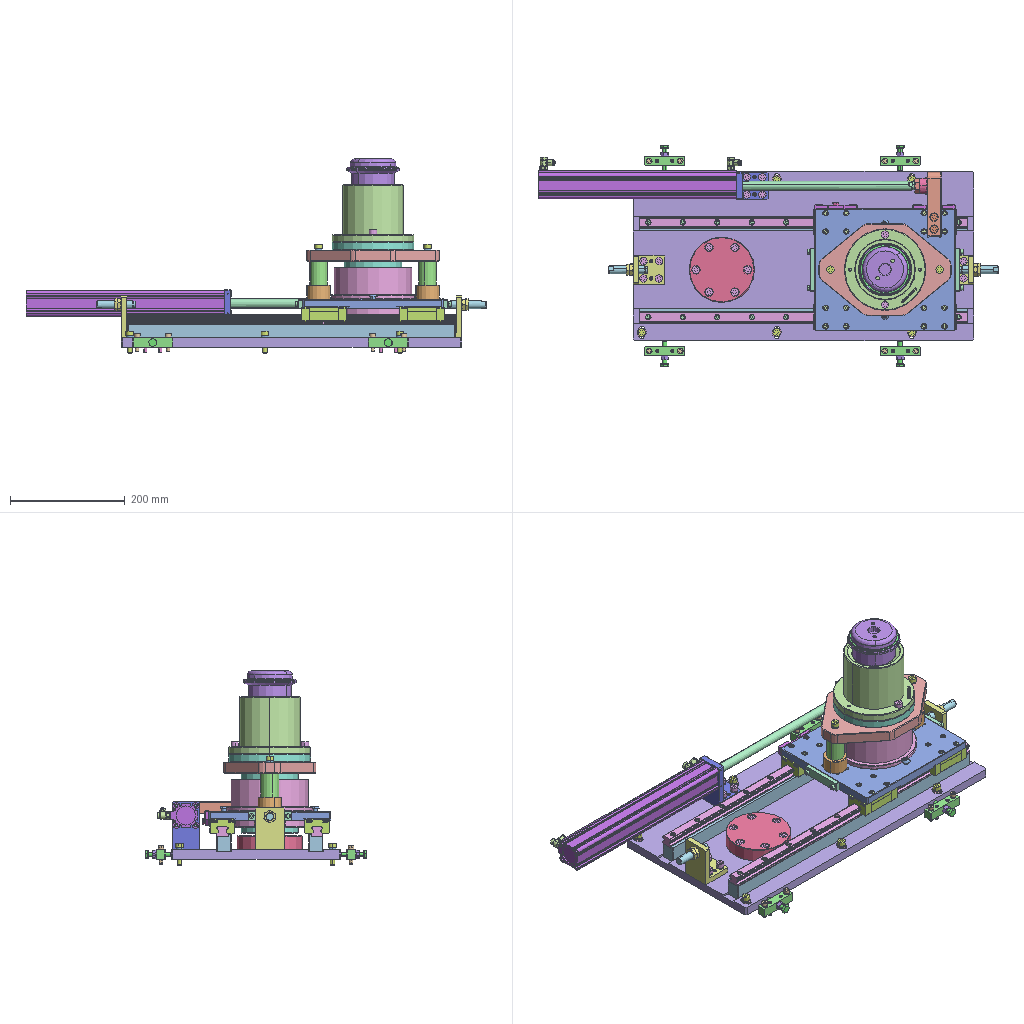Assembly | SolidWorks | 63 different items | 324 placed | box 801 x 386 x 338 mm
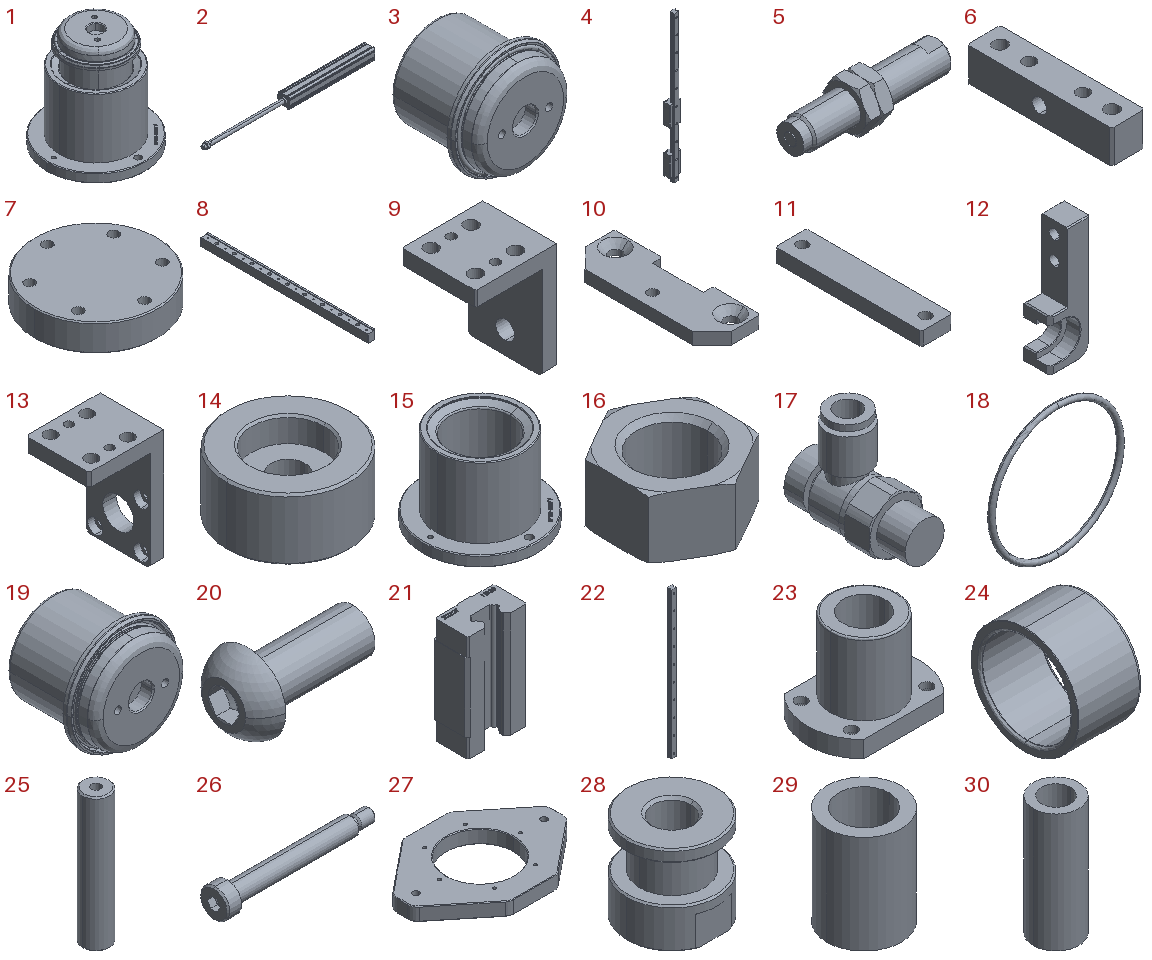Parts list (item | name | quantity | parent item | size | volume | features):
1 | (subassembly) | x1 | - | 142 x 142 x 150.5 mm | 760859 mm3 | -
2 | (subassembly) | x1 | - | 676 x 49.5 x 45 mm | 398264 mm3 | -
3 | (subassembly) | x1 | in 1 | 92 x 83 x 92 mm | 149578 mm3 | -
4 | (subassembly) | x2 | - | 44 x 30 x 570 mm | 296416 mm3 | -
5 | (subassembly) | x2 | - | 67.1 x 21.939 x 19.79 mm | 12290 mm3 | -
6 | - | x4 | - | 16 x 70 x 16 mm | 15307 mm3 | features HoleWzd 3, Chamfer 1, ExtruThin 1
7 | - | x1 | - | 114 x 114 x 25 mm | 237134 mm3 | features Chamfer 1, CirPattern 1, Extrusion 1, HoleWzd 1
8 | - | x2 | - | 25 x 570 x 30 mm | 386551 mm3 | features Chamfer 2, HoleWzd 2, Extrusion 1, ICE 1, LPattern 1
9 | - | x2 | - | 55 x 50 x 73 mm | 54613 mm3 | features HoleWzd 3, Chamfer 2, Extrusion 1, ICE 1
10 | - | x2 | - | 25 x 75 x 6 mm | 9049 mm3 | features Chamfer 3, HoleWzd 2, ExtruThin 1, ICE 1
11 | - | x2 | - | 16 x 75 x 7 mm | 8053 mm3 | features Chamfer 1, Extrusion 1, HoleWzd 1
12 | - | x1 | - | 36 x 24 x 110 mm | 50408 mm3 | features Chamfer 7, ICE 3, Extrusion 1, Fillet 1, HoleWzd 1
13 | - | x1 | - | 55 x 47 x 84 mm | 50700 mm3 | features HoleWzd 3, Chamfer 2, ICE 2, CirPattern 1, Extrusion 1
14 | - | x1 | in 1 | 30 x 30 x 15 mm | 8651 mm3 | features Chamfer 2, ICE 2, Extrusion 1
15 | - | x1 | in 1 | 142 x 142 x 106 mm | 593458 mm3 | features ICE 5, Chamfer 4, Fillet 3, HoleWzd 3, Extrusion 1, RevCut 1
16 | - | x4 | - | 12.482 x 14.38 x 6.8 mm | 562.42 mm3 | features Cut 2, Chamfer 1, Extrusion 1
17 | - | x2 | - | 13 x 29.2 x 26.1 mm | 3843 mm3 | features BaseBody 1
18 | - | x1 | in 3 | 86.03 x 3.53 x 86.03 mm | 2537 mm3 | features RefAxis 1, Revolution 1
19 | - | x1 | in 3 | 92 x 83 x 92 mm | 147042 mm3 | features Fillet 7, ICE 5, Chamfer 3, RevCut 3, CirPattern 1, Revolution 1
20 | - | x2 | - | 24.4 x 14 x 14 mm | 1421 mm3 | features RevCut 2, Revolution 2, Cut 1, LPattern 1, RefAxis 1
21 | - | x4 | in 4 | 44 x 25.4 x 77.8 mm | 67305 mm3 | features BaseBody 1
22 | - | x2 | in 4 | 20 x 17.5 x 570 mm | 161806 mm3 | features ICE 2, BaseBody 1, HoleWzd 1, LPattern 1
23 | - | x2 | - | 54 x 38 x 42 mm | 27501 mm3 | features BaseBody 1
24 | - | x1 | - | 70 x 120 x 120 mm | 240473 mm3 | features BaseBody 1
25 | - | x2 | - | 20 x 20 x 100 mm | 29690 mm3 | features Chamfer 2, HoleWzd 2, Extrusion 1
26 | - | x1 | in 1 | 70 x 13 x 13 mm | 3701 mm3 | features BaseBody 1
27 | - | x1 | - | 230 x 160 x 20 mm | 361707 mm3 | features Chamfer 3, HoleWzd 2, ICE 2, Cut 1, Extrusion 1, Fillet 1
28 | - | x1 | - | 29.5 x 29.5 x 29 mm | 12018 mm3 | features BaseBody 1
29 | - | x2 | - | 31 x 31 x 41 mm | 16745 mm3 | features Extrusion 1
30 | - | x1 | in 1 | 16.5 x 16.5 x 43 mm | 5471 mm3 | features Extrusion 1, ICE 1
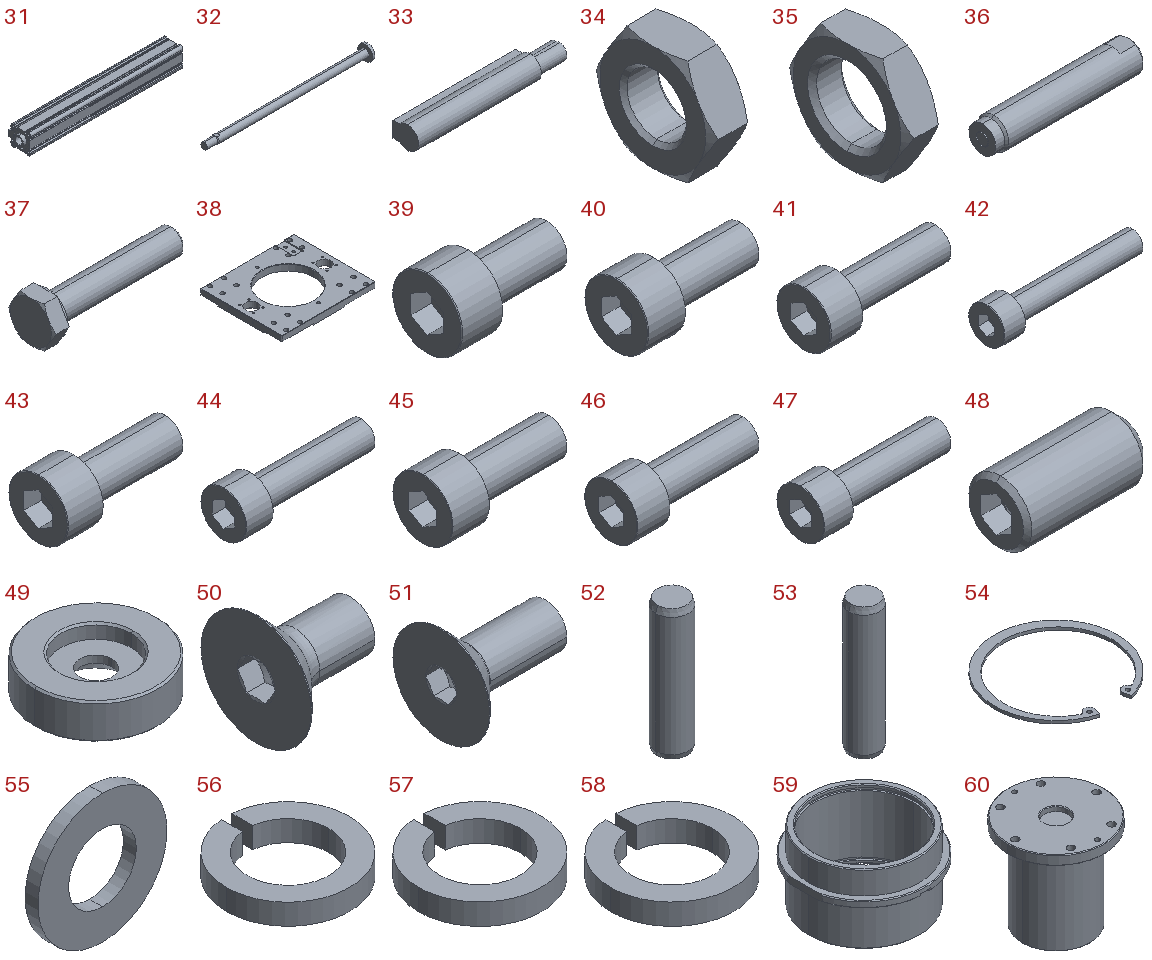31 | - | x1 | in 2 | 350.5 x 49.5 x 45 mm | 322350 mm3 | features BaseBody 1
32 | - | x1 | in 2 | 353.5 x 32 x 32 mm | 72863 mm3 | features BaseBody 1
33 | - | x2 | in 2 | 27 x 4.6 x 4 mm | 354.995 mm3 | features BaseBody 1
34 | - | x1 | in 2 | 8 x 25.403 x 22 mm | 2341 mm3 | features BaseBody 1
35 | - | x4 | in 5 | 6 x 21.939 x 19 mm | 1112 mm3 | features BaseBody 1
36 | - | x2 | in 5 | 67.1 x 14 x 14 mm | 10065 mm3 | features BaseBody 1
37 | - | x4 | - | 45.3 x 15.011 x 13 mm | 2765 mm3 | features RevCut 4, Chamfer 1, Extrusion 1, Fillet 1, LPattern 1, Revolution 1
38 | - | x1 | - | 245 x 213 x 16 mm | 513654 mm3 | features HoleWzd 7, Chamfer 4, ICE 3, Cut 2, Extrusion 1, Fillet 1
39 | - | x8 | - | 15 x 8.5 x 8.5 mm | 444.118 mm3 | features BlendCut 1, Cut 1, Fillet 1, LPattern 1, RevCut 1, Revolution 1
40 | - | x16 | - | 17 x 8.5 x 8.5 mm | 483.388 mm3 | features BlendCut 1, Cut 1, Fillet 1, LPattern 1, RevCut 1, Revolution 1
41 | - | x30 | - | 21 x 8.5 x 8.5 mm | 561.928 mm3 | features BlendCut 1, Cut 1, Fillet 1, LPattern 1, RevCut 1, Revolution 1
42 | - | x18 | - | 35 x 8.5 x 8.5 mm | 836.817 mm3 | features BlendCut 1, Cut 1, Fillet 1, LPattern 1, RevCut 1, Revolution 1
43 | - | x4 | - | 22 x 10 x 10 mm | 856.284 mm3 | features BlendCut 1, Cut 1, Fillet 1, LPattern 1, RevCut 1, Revolution 1
44 | - | x8 | - | 31 x 10 x 10 mm | 1111 mm3 | features BlendCut 1, Cut 1, Fillet 1, LPattern 1, RevCut 1, Revolution 1
45 | - | x2 | - | 28 x 13 x 13 mm | 1937 mm3 | features BlendCut 1, Cut 1, Fillet 1, LPattern 1, RevCut 1, Revolution 1
46 | - | x20 | - | 33 x 13 x 13 mm | 2189 mm3 | features BlendCut 1, Cut 1, Fillet 1, LPattern 1, RevCut 1, Revolution 1
47 | - | x8 | - | 38 x 13 x 13 mm | 2440 mm3 | features BlendCut 1, Cut 1, Fillet 1, LPattern 1, RevCut 1, Revolution 1
48 | - | x2 | - | 12 x 6 x 6 mm | 312.089 mm3 | features RevCut 2, Cut 1, LPattern 1, Revolution 1
49 | - | x2 | - | 35 x 35 x 10 mm | 7654 mm3 | features Chamfer 2, Extrusion 1, HoleWzd 1, ICE 1
50 | - | x4 | - | 12 x 13.44 x 13.44 mm | 493.143 mm3 | features RevCut 2, Revolution 2, Cut 1, LPattern 1, RefAxis 1
51 | - | x2 | - | 20 x 17.92 x 17.92 mm | 1375 mm3 | features RevCut 2, Revolution 2, Cut 1, LPattern 1, RefAxis 1
52 | - | x6 | - | 6 x 6 x 24 mm | 569.991 mm3 | features Chamfer 3, Cut 2, Extrusion 1, RevCut 1
53 | - | x8 | - | 6 x 6 x 26 mm | 626.54 mm3 | features Chamfer 3, Cut 2, Extrusion 1, RevCut 1
54 | - | x2 | - | 127 x 124.836 x 3 mm | 7725 mm3 | features Extrusion 1
55 | - | x6 | - | 16 x 1.6 x 16 mm | 233.031 mm3 | features Revolution 1
56 | - | x64 | - | 7.686 x 7.672 x 1.3 mm | 32.664 mm3 | features Extrusion 1
57 | - | x12 | - | 9.282 x 9.265 x 1.6 mm | 59.463 mm3 | features Extrusion 1
58 | - | x28 | - | 12.277 x 12.254 x 2.1 mm | 135.755 mm3 | features Extrusion 1
59 | - | x1 | - | 144 x 150 x 84 mm | 271588 mm3 | features ICE 4, Chamfer 1, Extrusion 1, RevCut 1
60 | - | x1 | - | 142 x 142 x 138 mm | 1182904 mm3 | features Chamfer 4, HoleWzd 2, ICE 2, CirPattern 1, Extrusion 1
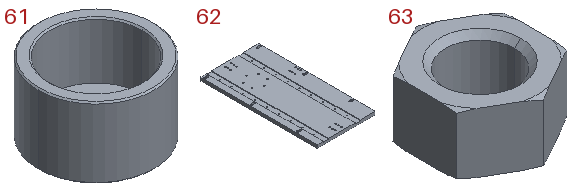61 | - | x2 | - | 41 x 41 x 25 mm | 14638 mm3 | features Chamfer 2, ICE 2, Extrusion 1
62 | - | x1 | - | 295 x 593 x 16 mm | 2656346 mm3 | features HoleWzd 6, ICE 2, Chamfer 1, Cut 1, Extrusion 1
63 | - | x2 | - | 9.591 x 11.05 x 5.2 mm | 259.734 mm3 | features Cut 2, Chamfer 1, Extrusion 1
Mates (type | each side: item.copy, entity, surface, feature), first 567 of 641 lines:
In the top assembly
Coincident | 27.1 plane | assembly plane | 4 times
Coincident | 59.1 face plane Cut-Revolve1 | 54.1 face plane Base-Extrude
Concentric | 59.1 face cylinder Cut-Revolve1 | 54.1 face cylinder Base-Extrude
Concentric | 59.1 face cylinder Boss-Extrude2 | 54.2 face cylinder Base-Extrude
Coincident | 59.1 face plane Cut-Revolve1 | 54.2 face plane Base-Extrude
Concentric | 59.1 face cylinder Boss-Extrude2 | 24.1 face cylinder Input1
Coincident | 59.1 face plane Cut-Revolve1 | 24.1 face plane Input1
Coincident | 38.1 face plane Boss-Extrude1 | 59.1 face plane Boss-Extrude1
Concentric | 38.1 face cylinder Cut-Extrude2 | 59.1 face cylinder Boss-Extrude2
Concentric | 24.1 face cylinder Input1 | 60.1 face cylinder Boss-Extrude1
Coincident | 27.1 face plane Boss-Extrude1 | 60.1 face plane Boss-Extrude2
Concentric | 38.1 face cylinder Cut-Extrude3 | 23.1 face cylinder Input1
Coincident | 38.1 face plane Boss-Extrude1 | 23.1 face plane Input1
Parallel | 38.1 face plane Boss-Extrude1 | 23.1 face plane Input1
Concentric | 38.1 face cylinder Cut-Extrude3 | 23.2 face cylinder Input1
Coincident | 38.1 face plane Boss-Extrude1 | 23.2 face plane Input1
Parallel | 38.1 face plane Boss-Extrude1 | 23.2 face plane Input1
Concentric | 27.1 face cylinder Cut-Extrude4 | 25.1 face cylinder Boss-Extrude1
Coincident | 27.1 face plane Cut-Extrude4 | 25.1 face plane Boss-Extrude1
Concentric | 27.1 face cylinder Cut-Extrude4 | 25.2 face cylinder Boss-Extrude1
Coincident | 27.1 face plane Cut-Extrude4 | 25.2 face plane Boss-Extrude1
Concentric | 23.2 face cylinder Input1 | 25.1 face cylinder Boss-Extrude1
Concentric | 23.1 face cylinder Input1 | 25.2 face cylinder Boss-Extrude1
Concentric | 49.1 face cylinder Cut-Extrude1 | 25.1 face cylinder Boss-Extrude1
Coincident | 49.1 face plane Cut-Extrude1 | 25.1 face plane Boss-Extrude1
Concentric | 49.2 face cylinder Boss-Extrude1 | 25.2 face cylinder Boss-Extrude1
Coincident | 49.2 face plane Cut-Extrude1 | 25.2 face plane Boss-Extrude1
Coincident | 49.1 face plane Boss-Extrude1 | 23.2 face plane Input1
Concentric | 60.1 face cylinder Boss-Extrude2 | 15.1 face cylinder Boss-Extrude1
Coincident | 60.1 face plane Boss-Extrude1 | 15.1 face plane Boss-Extrude1
Concentric | 25.2 face cylinder Boss-Extrude1 | 61.1 face cylinder Boss-Extrude1
Coincident | 38.1 face plane Boss-Extrude1 | 61.1 face plane Boss-Extrude1
Concentric | 23.2 face cylinder Input1 | 61.2 face cylinder Boss-Extrude1
Coincident | 38.1 face plane Boss-Extrude1 | 61.2 face plane Boss-Extrude1
Concentric | 25.2 face cylinder Boss-Extrude1 | 29.1 face cylinder Boss-Extrude1
Coincident | 61.1 face plane Boss-Extrude1 | 29.1 face plane Boss-Extrude1
Concentric | 25.1 face cylinder Boss-Extrude1 | 29.2 face cylinder Boss-Extrude1
Coincident | 61.2 face plane Boss-Extrude1 | 29.2 face plane Boss-Extrude1
DistanceDim | 21.1 face plane Input1 | 38.1 face plane Boss-Extrude1 | 2 times
Width | 21.1 face plane Input1 | 21.2 face plane Input1 | 38.1 face plane Boss-Extrude1 | 38.1 face plane Boss-Extrude1
Coincident | 22.1 face plane Input1 | 22.2 face plane Input1 | 2 times
DistanceDim | 21.3 face plane Input1 | 38.1 face plane Boss-Extrude1
Coincident | 21.1 face plane Input1 | 21.3 face plane Input1
Coincident | 22.2 face plane Input1 | 8.1 face plane Extrude1 | 2 times
Coincident | 22.2 face plane Input1 | 8.1 face plane Cut-Extrude1 | 2 times
Coincident | 22.1 face plane Input1 | 8.2 face plane Cut-Extrude1 | 2 times
Coincident | 8.1 face plane Extrude1 | 8.2 face plane Extrude1
Coincident | 62.1 face plane Cut-Extrude1 | 8.1 face plane Extrude1 | 2 times
Coincident | 62.1 face plane Extrude1 | 9.1 face plane Boss-Extrude1
DistanceDim | 62.1 face plane Extrude1 | 9.1 face plane Boss-Extrude1
Coincident | 62.1 face plane Extrude1 | 6.1 face plane Extrude-Thin1
DistanceDim | 6.1 face plane Extrude-Thin1 | 62.1 face plane Extrude1
DistanceDim | 62.1 face plane Extrude1 | 6.1 face plane Extrude-Thin1
Coincident | 38.1 face plane Boss-Extrude1 | 10.1 face plane Extrude-Thin1
Width | 10.1 face plane Extrude-Thin1 | 10.1 face plane Extrude-Thin1 | 21.2 face plane Input1 | 21.2 face plane Input1
DistanceDim | 38.1 face plane Boss-Extrude1 | 10.1 face plane Extrude-Thin1
Coincident | 38.1 face plane Boss-Extrude1 | 10.2 face plane Extrude-Thin1
DistanceDim | 10.2 face plane Extrude-Thin1 | 38.1 face plane Boss-Extrude1
Width | 10.2 face plane Extrude-Thin1 | 10.2 face plane Extrude-Thin1 | 21.1 face plane Input1 | 21.1 face plane Input1
Concentric | 9.1 face cylinder M14x1.5 Tapped Hole1 | 36.1 face cylinder Input1
Coincident | 27.1 plane | 60.1 plane
Parallel | 27.1 face plane Boss-Extrude1 | 1.1 plane
Parallel | 38.1 face plane Boss-Extrude1 | 59.1 face plane Cut-Extrude2
Concentric | 38.1 face cylinder M8 Tapped Hole1 | 20.1 face cylinder Revolve1
Coincident | 59.1 face plane Cut-Extrude3 | 20.1 face plane Revolve1
Concentric | 38.1 face cylinder M8 Tapped Hole1 | 20.2 face cylinder Revolve1
Coincident | 59.1 face plane Cut-Extrude3 | 20.2 face plane Revolve1
Coincident | 38.1 face plane Boss-Extrude1 | 11.1 face plane Boss-Extrude1 | 2 times
Width | 11.1 face plane Boss-Extrude1 | 11.1 face plane Boss-Extrude1 | 22.1 face plane Input1 | 22.2 face plane Input1
Coincident | 38.1 face plane Boss-Extrude1 | 11.2 face plane Boss-Extrude1 | 2 times
Coincident | 11.1 face plane Boss-Extrude1 | 11.2 face plane Boss-Extrude1
Coincident | 9.1 face plane Boss-Extrude1 | 35.1 face plane Input1
Coincident | 62.1 face plane Extrude1 | 9.2 face plane Boss-Extrude1 | 2 times
Coincident | 9.1 face plane Boss-Extrude1 | 9.2 face plane Boss-Extrude1
Concentric | 36.2 face cylinder Input1 | 9.2 face cylinder M14x1.5 Tapped Hole1
Coincident | 35.2 face plane Input1 | 9.2 face plane Boss-Extrude1
Width | 9.1 face plane Boss-Extrude1 | 9.1 face plane Boss-Extrude1 | 22.1 face plane Input1 | 22.2 face plane Input1
DistanceDim | 8.1 face plane Extrude1 | 62.1 face plane Extrude1
Coincident | 6.1 face plane Extrude-Thin1 | 6.2 face plane Extrude-Thin1 | 2 times
DistanceDim | 6.3 face plane Extrude-Thin1 | 62.1 face plane Extrude1
Coincident | 62.1 face plane Extrude1 | 6.3 face plane Extrude-Thin1
Coincident | 6.1 face plane Extrude-Thin1 | 6.3 face plane Extrude-Thin1
Coincident | 6.3 face plane Extrude-Thin1 | 6.4 face plane Extrude-Thin1 | 2 times
Coincident | 6.2 face plane Extrude-Thin1 | 6.4 face plane Extrude-Thin1
DistanceDim | 6.2 face plane Extrude-Thin1 | 62.1 face plane Extrude1
Coincident | 62.1 face plane Extrude1 | 7.1 face plane Boss-Extrude1
DistanceDim | 7.1 plane | 62.1 face plane Extrude1
DistanceDim | 7.1 plane | 62.1 face plane Cut-Extrude1
Coincident | 38.1 face plane Cut-Extrude5 | 12.1 face plane Boss-Extrude1
Coincident | 62.1 face plane Extrude1 | 13.1 face plane Boss-Extrude1
DistanceDim | 13.1 face plane Boss-Extrude1 | 62.1 face plane Extrude1 | 2 times
Coincident | 13.1 face plane Boss-Extrude1 | 31.1 face plane Input1
Concentric | 13.1 face cylinder Cut-Extrude1 | 31.1 face cylinder Input1
Concentric | 13.1 face cylinder CirPattern1 | 31.1 face cylinder Input1
Concentric | 32.1 face cylinder Input1 | 28.1 face cylinder Input1
Coincident | 34.1 face plane Input1 | 28.1 face plane Input1
DistanceDim | 38.1 face plane Cut-Extrude5 | 12.1 face plane Boss-Extrude1
Concentric | 31.1 face cylinder Input1 | 17.1 face cylinder Input1
DistanceDim | 17.1 face plane Input1 | 31.1 face plane Input1
Concentric | 31.1 face cylinder Input1 | 17.2 face cylinder Input1
DistanceDim | 17.2 face plane Input1 | 31.1 face plane Input1
Coincident | 12.1 face plane Cut-Extrude2 | 28.1 face plane Input1
DistanceDim | 12.1 face plane Boss-Extrude1 | 38.1 face plane Boss-Extrude1
Concentric | 6.4 face cylinder Size mm blind dowel hole 1 | 53.1 face cylinder Base-Extrude
Coincident | 6.4 face plane Extrude-Thin1 | 53.1 face plane Base-Extrude
Concentric | 6.4 face cylinder Size mm blind dowel hole 1 | 53.2 face cylinder Base-Extrude
Coincident | 6.4 face plane Extrude-Thin1 | 53.2 face plane Base-Extrude
Concentric | 6.3 face cylinder Size mm blind dowel hole 1 | 53.3 face cylinder Base-Extrude
Coincident | 6.3 face plane Extrude-Thin1 | 53.3 face plane Base-Extrude
Concentric | 6.3 face cylinder Size mm blind dowel hole 1 | 53.4 face cylinder Base-Extrude
Coincident | 6.3 face plane Extrude-Thin1 | 53.4 face plane Base-Extrude
Concentric | 6.1 face cylinder Size mm blind dowel hole 1 | 53.5 face cylinder Base-Extrude
Coincident | 6.1 face plane Extrude-Thin1 | 53.5 face plane Base-Extrude
Concentric | 6.1 face cylinder Size mm blind dowel hole 1 | 53.6 face cylinder Base-Extrude
Coincident | 6.1 face plane Extrude-Thin1 | 53.6 face plane Base-Extrude
Concentric | 6.2 face cylinder Size mm blind dowel hole 1 | 53.7 face cylinder Base-Extrude
Coincident | 6.2 face plane Extrude-Thin1 | 53.7 face plane Base-Extrude
Concentric | 6.2 face cylinder Size mm blind dowel hole 1 | 53.8 face cylinder Base-Extrude
Coincident | 6.2 face plane Extrude-Thin1 | 53.8 face plane Base-Extrude
Coincident | 6.3 face plane Extrude-Thin1 | 57.1 face plane Extrude1
Concentric | 6.3 face cylinder M6 Clearance Hole1 | 57.1 face cylinder Extrude1
Coincident | 6.3 face plane Extrude-Thin1 | 57.2 face plane Extrude1
Concentric | 6.3 face cylinder M6 Clearance Hole1 | 57.2 face cylinder Extrude1
Coincident | 6.4 face plane Extrude-Thin1 | 57.3 face plane Extrude1
Concentric | 6.4 face cylinder M6 Clearance Hole1 | 57.3 face cylinder Extrude1
Coincident | 6.4 face plane Extrude-Thin1 | 57.4 face plane Extrude1
Concentric | 6.4 face cylinder M6 Clearance Hole1 | 57.4 face cylinder Extrude1
Coincident | 6.2 face plane Extrude-Thin1 | 57.5 face plane Extrude1
Concentric | 6.2 face cylinder M6 Clearance Hole1 | 57.5 face cylinder Extrude1
Coincident | 6.2 face plane Extrude-Thin1 | 57.6 face plane Extrude1
Concentric | 6.2 face cylinder M6 Clearance Hole1 | 57.6 face cylinder Extrude1
Coincident | 6.1 face plane Extrude-Thin1 | 57.7 face plane Extrude1
Concentric | 6.1 face cylinder M6 Clearance Hole1 | 57.7 face cylinder Extrude1
Coincident | 6.1 face plane Extrude-Thin1 | 57.8 face plane Extrude1
Concentric | 6.1 face cylinder M6 Clearance Hole1 | 57.8 face cylinder Extrude1
Coincident | 57.8 face plane Extrude1 | 44.1 face plane Base-Revolve
Concentric | 57.8 face cylinder Extrude1 | 44.1 face cylinder Base-Revolve
Coincident | 57.7 face plane Extrude1 | 44.2 face plane Base-Revolve
Concentric | 57.7 face cylinder Extrude1 | 44.2 face cylinder Base-Revolve
Coincident | 57.6 face plane Extrude1 | 44.3 face plane Base-Revolve
Concentric | 57.6 face cylinder Extrude1 | 44.3 face cylinder Base-Revolve
Coincident | 57.5 face plane Extrude1 | 44.4 face plane Base-Revolve
Concentric | 57.5 face cylinder Extrude1 | 44.4 face cylinder Base-Revolve
Coincident | 57.4 face plane Extrude1 | 44.5 face plane Base-Revolve
Concentric | 57.4 face cylinder Extrude1 | 44.5 face cylinder Base-Revolve
Coincident | 57.3 face plane Extrude1 | 44.6 face plane Base-Revolve
Concentric | 57.3 face cylinder Extrude1 | 44.6 face cylinder Base-Revolve
Coincident | 57.2 face plane Extrude1 | 44.7 face plane Base-Revolve
Concentric | 57.2 face cylinder Extrude1 | 44.7 face cylinder Base-Revolve
Coincident | 57.1 face plane Extrude1 | 44.8 face plane Base-Revolve
Concentric | 57.1 face cylinder Extrude1 | 44.8 face cylinder Base-Revolve
Concentric | 6.3 face cylinder M8 Tapped Hole1 | 16.1 face cylinder Base-Extrude
Coincident | 6.3 face plane Extrude-Thin1 | 16.1 face plane Base-Extrude
Concentric | 6.4 face cylinder M8 Tapped Hole1 | 16.2 face cylinder Base-Extrude
Coincident | 6.4 face plane Extrude-Thin1 | 16.2 face plane Base-Extrude
Concentric | 6.2 face cylinder M8 Tapped Hole1 | 16.3 face cylinder Base-Extrude
Coincident | 6.2 face plane Extrude-Thin1 | 16.3 face plane Base-Extrude
Concentric | 6.1 face cylinder M8 Tapped Hole1 | 16.4 face cylinder Base-Extrude
Coincident | 6.1 face plane Extrude-Thin1 | 16.4 face plane Base-Extrude
Concentric | 16.4 face cylinder Base-Extrude | 37.1 face cylinder Boss-Revolve1
Coincident | 62.1 face plane Extrude1 | 37.1 face plane Boss-Revolve1
Concentric | 16.3 face cylinder Base-Extrude | 37.2 face cylinder Boss-Revolve1
Coincident | 62.1 face plane Extrude1 | 37.2 face plane Boss-Revolve1
Concentric | 16.2 face cylinder Base-Extrude | 37.3 face cylinder Boss-Revolve1
Coincident | 62.1 face plane Extrude1 | 37.3 face plane Boss-Revolve1
Concentric | 16.1 face cylinder Base-Extrude | 37.4 face cylinder Boss-Revolve1
Coincident | 62.1 face plane Extrude1 | 37.4 face plane Boss-Revolve1
Coincident | 62.1 face plane Extrude1 | 55.1 face plane Base-Revolve
Concentric | 62.1 face cylinder Cut-Extrude3 | 55.1 face cylinder Base-Revolve
Coincident | 62.1 face plane Extrude1 | 55.2 face plane Base-Revolve
Concentric | 62.1 face cylinder Cut-Extrude3 | 55.2 face cylinder Base-Revolve
Coincident | 62.1 face plane Extrude1 | 55.3 face plane Base-Revolve
Concentric | 62.1 face cylinder Cut-Extrude3 | 55.3 face cylinder Base-Revolve
Coincident | 62.1 face plane Extrude1 | 55.4 face plane Base-Revolve
Concentric | 62.1 face cylinder Cut-Extrude3 | 55.4 face cylinder Base-Revolve
Coincident | 62.1 face plane Extrude1 | 55.5 face plane Base-Revolve
Concentric | 62.1 face cylinder Cut-Extrude3 | 55.5 face cylinder Base-Revolve
Coincident | 62.1 face plane Extrude1 | 55.6 face plane Base-Revolve
Concentric | 62.1 face cylinder Cut-Extrude3 | 55.6 face cylinder Base-Revolve
Coincident | 55.6 face plane Base-Revolve | 58.1 face plane Extrude1
Concentric | 55.6 face cylinder Base-Revolve | 58.1 face cylinder Extrude1
Coincident | 55.5 face plane Base-Revolve | 58.2 face plane Extrude1
Concentric | 55.5 face cylinder Base-Revolve | 58.2 face cylinder Extrude1
Coincident | 55.4 face plane Base-Revolve | 58.3 face plane Extrude1
Concentric | 55.4 face cylinder Base-Revolve | 58.3 face cylinder Extrude1
Coincident | 58.3 face plane Extrude1 | 47.1 face plane Base-Revolve
Concentric | 58.3 face cylinder Extrude1 | 47.1 face cylinder Base-Revolve
Coincident | 58.2 face plane Extrude1 | 47.2 face plane Base-Revolve
Concentric | 58.2 face cylinder Extrude1 | 47.2 face cylinder Base-Revolve
Coincident | 58.1 face plane Extrude1 | 47.3 face plane Base-Revolve
Concentric | 58.1 face cylinder Extrude1 | 47.3 face cylinder Base-Revolve
Coincident | 55.1 face plane Base-Revolve | 58.4 face plane Extrude1
Concentric | 55.1 face cylinder Base-Revolve | 58.4 face cylinder Extrude1
Coincident | 55.2 face plane Base-Revolve | 58.5 face plane Extrude1
Concentric | 55.2 face cylinder Base-Revolve | 58.5 face cylinder Extrude1
Coincident | 55.3 face plane Base-Revolve | 58.6 face plane Extrude1
Concentric | 55.3 face cylinder Base-Revolve | 58.6 face cylinder Extrude1
Coincident | 58.4 face plane Extrude1 | 47.4 face plane Base-Revolve
Concentric | 58.4 face cylinder Extrude1 | 47.4 face cylinder Base-Revolve
Coincident | 58.5 face plane Extrude1 | 47.5 face plane Base-Revolve
Concentric | 58.5 face cylinder Extrude1 | 47.5 face cylinder Base-Revolve
Coincident | 58.6 face plane Extrude1 | 47.6 face plane Base-Revolve
Concentric | 58.6 face cylinder Extrude1 | 47.6 face cylinder Base-Revolve
Coincident | 13.1 face plane Boss-Extrude1 | 58.7 face plane Extrude1
Concentric | 13.1 face cylinder M8 Clearance Hole1 | 58.7 face cylinder Extrude1
Coincident | 13.1 face plane Boss-Extrude1 | 58.8 face plane Extrude1
Concentric | 13.1 face cylinder M8 Clearance Hole1 | 58.8 face cylinder Extrude1
Coincident | 13.1 face plane Boss-Extrude1 | 58.9 face plane Extrude1
Concentric | 13.1 face cylinder M8 Clearance Hole1 | 58.9 face cylinder Extrude1
Coincident | 13.1 face plane Boss-Extrude1 | 58.10 face plane Extrude1
Concentric | 13.1 face cylinder M8 Clearance Hole1 | 58.10 face cylinder Extrude1
Coincident | 58.7 face plane Extrude1 | 46.1 face plane Base-Revolve
Concentric | 58.7 face cylinder Extrude1 | 46.1 face cylinder Base-Revolve
Coincident | 58.8 face plane Extrude1 | 46.2 face plane Base-Revolve
Concentric | 58.8 face cylinder Extrude1 | 46.2 face cylinder Base-Revolve
Coincident | 58.9 face plane Extrude1 | 46.3 face plane Base-Revolve
Concentric | 58.9 face cylinder Extrude1 | 46.3 face cylinder Base-Revolve
Coincident | 58.10 face plane Extrude1 | 46.4 face plane Base-Revolve
Concentric | 58.10 face cylinder Extrude1 | 46.4 face cylinder Base-Revolve
Concentric | 13.1 face cylinder Size mm blind dowel hole 1 | 52.1 face cylinder Base-Extrude
Coincident | 13.1 face plane Boss-Extrude1 | 52.1 face plane Base-Extrude
Concentric | 13.1 face cylinder Size mm blind dowel hole 1 | 52.2 face cylinder Base-Extrude
Coincident | 13.1 face plane Boss-Extrude1 | 52.2 face plane Base-Extrude
Coincident | 9.1 face plane Boss-Extrude1 | 58.11 face plane Extrude1
Concentric | 9.1 face cylinder M8 Clearance Hole1 | 58.11 face cylinder Extrude1
Coincident | 9.1 face plane Boss-Extrude1 | 58.12 face plane Extrude1
Concentric | 9.1 face cylinder M8 Clearance Hole1 | 58.12 face cylinder Extrude1
Coincident | 9.1 face plane Boss-Extrude1 | 58.13 face plane Extrude1
Concentric | 9.1 face cylinder M8 Clearance Hole1 | 58.13 face cylinder Extrude1
Coincident | 9.1 face plane Boss-Extrude1 | 58.14 face plane Extrude1
Concentric | 9.1 face cylinder M8 Clearance Hole1 | 58.14 face cylinder Extrude1
Coincident | 9.2 face plane Boss-Extrude1 | 58.15 face plane Extrude1
Concentric | 9.2 face cylinder M8 Clearance Hole1 | 58.15 face cylinder Extrude1
Coincident | 9.2 face plane Boss-Extrude1 | 58.16 face plane Extrude1
Concentric | 9.2 face cylinder M8 Clearance Hole1 | 58.16 face cylinder Extrude1
Coincident | 9.2 face plane Boss-Extrude1 | 58.17 face plane Extrude1
Concentric | 9.2 face cylinder M8 Clearance Hole1 | 58.17 face cylinder Extrude1
Coincident | 9.2 face plane Boss-Extrude1 | 58.18 face plane Extrude1
Concentric | 9.2 face cylinder M8 Clearance Hole1 | 58.18 face cylinder Extrude1
Coincident | 58.13 face plane Extrude1 | 46.5 face plane Base-Revolve
Concentric | 9.1 face cylinder M8 Clearance Hole1 | 46.5 face cylinder Base-Revolve
Coincident | 58.11 face plane Extrude1 | 46.6 face plane Base-Revolve
Concentric | 58.11 face cylinder Extrude1 | 46.6 face cylinder Base-Revolve
Coincident | 58.12 face plane Extrude1 | 46.7 face plane Base-Revolve
Concentric | 58.12 face cylinder Extrude1 | 46.7 face cylinder Base-Revolve
Coincident | 58.14 face plane Extrude1 | 46.8 face plane Base-Revolve
Concentric | 58.14 face cylinder Extrude1 | 46.8 face cylinder Base-Revolve
Coincident | 58.16 face plane Extrude1 | 46.9 face plane Base-Revolve
Concentric | 58.16 face cylinder Extrude1 | 46.9 face cylinder Base-Revolve
Coincident | 58.18 face plane Extrude1 | 46.10 face plane Base-Revolve
Concentric | 58.18 face cylinder Extrude1 | 46.10 face cylinder Base-Revolve
Coincident | 58.15 face plane Extrude1 | 46.11 face plane Base-Revolve
Concentric | 58.15 face cylinder Extrude1 | 46.11 face cylinder Base-Revolve
Coincident | 58.17 face plane Extrude1 | 46.12 face plane Base-Revolve
Concentric | 58.17 face cylinder Extrude1 | 46.12 face cylinder Base-Revolve
Concentric | 9.1 face cylinder Size mm blind dowel hole 1 | 52.3 face cylinder Base-Extrude
Coincident | 9.1 face plane Boss-Extrude1 | 52.3 face plane Base-Extrude
Concentric | 9.1 face cylinder Size mm blind dowel hole 1 | 52.4 face cylinder Base-Extrude
Coincident | 9.1 face plane Boss-Extrude1 | 52.4 face plane Base-Extrude
Concentric | 9.2 face cylinder Size mm blind dowel hole 1 | 52.5 face cylinder Base-Extrude
Coincident | 9.2 face plane Boss-Extrude1 | 52.5 face plane Base-Extrude
Concentric | 9.2 face cylinder Size mm blind dowel hole 1 | 52.6 face cylinder Base-Extrude
Coincident | 9.2 face plane Boss-Extrude1 | 52.6 face plane Base-Extrude
Coincident | 7.1 face plane Hole size (per socket head cap screw type)1 | 58.19 face plane Extrude1
Concentric | 7.1 face cylinder Hole size (per socket head cap screw type)1 | 58.19 face cylinder Extrude1
Coincident | 7.1 face plane CirPattern1 | 58.20 face plane Extrude1
Concentric | 7.1 face cylinder CirPattern1 | 58.20 face cylinder Extrude1
Coincident | 7.1 face plane CirPattern1 | 58.21 face plane Extrude1
Concentric | 7.1 face cylinder CirPattern1 | 58.21 face cylinder Extrude1
Coincident | 7.1 face plane CirPattern1 | 58.22 face plane Extrude1
Concentric | 7.1 face cylinder CirPattern1 | 58.22 face cylinder Extrude1
Coincident | 7.1 face plane CirPattern1 | 58.23 face plane Extrude1
Concentric | 7.1 face cylinder CirPattern1 | 58.23 face cylinder Extrude1
Coincident | 7.1 face plane CirPattern1 | 58.24 face plane Extrude1
Concentric | 7.1 face cylinder CirPattern1 | 58.24 face cylinder Extrude1
Coincident | 58.24 face plane Extrude1 | 46.13 face plane Base-Revolve
Concentric | 7.1 face cylinder CirPattern1 | 46.13 face cylinder Base-Revolve
Coincident | 58.19 face plane Extrude1 | 46.14 face plane Base-Revolve
Concentric | 7.1 face cylinder Hole size (per socket head cap screw type)1 | 46.14 face cylinder Base-Revolve
Coincident | 58.20 face plane Extrude1 | 46.15 face plane Base-Revolve
Concentric | 7.1 face cylinder CirPattern1 | 46.15 face cylinder Base-Revolve
Coincident | 58.21 face plane Extrude1 | 46.16 face plane Base-Revolve
Concentric | 7.1 face cylinder CirPattern1 | 46.16 face cylinder Base-Revolve
Coincident | 58.22 face plane Extrude1 | 46.17 face plane Base-Revolve
Concentric | 7.1 face cylinder CirPattern1 | 46.17 face cylinder Base-Revolve
Coincident | 58.23 face plane Extrude1 | 46.18 face plane Base-Revolve
Concentric | 7.1 face cylinder CirPattern1 | 46.18 face cylinder Base-Revolve
Coincident | 12.1 face plane Hole size (per socket head cap screw type)2 | 58.25 face plane Extrude1
Concentric | 12.1 face cylinder Hole size (per socket head cap screw type)2 | 58.25 face cylinder Extrude1
Coincident | 12.1 face plane Hole size (per socket head cap screw type)2 | 58.26 face plane Extrude1
Concentric | 12.1 face cylinder Hole size (per socket head cap screw type)2 | 58.26 face cylinder Extrude1
Coincident | 58.25 face plane Extrude1 | 45.1 face plane Base-Revolve
Concentric | 12.1 face cylinder Hole size (per socket head cap screw type)2 | 45.1 face cylinder Base-Revolve
Coincident | 58.26 face plane Extrude1 | 45.2 face plane Base-Revolve
Concentric | 12.1 face cylinder Hole size (per socket head cap screw type)2 | 45.2 face cylinder Base-Revolve
Concentric | 10.1 face cylinder Hole size (per socket flat counteREDACTEDk head screw type)1 | 50.1 face cylinder Revolve1
DistanceDim | 50.1 face plane Revolve1 | 10.1 face plane Extrude-Thin1
Concentric | 10.1 face cylinder Hole size (per socket flat counteREDACTEDk head screw type)1 | 50.2 face cylinder Revolve1
DistanceDim | 50.2 face plane Revolve1 | 10.1 face plane Extrude-Thin1
Concentric | 10.2 face cylinder Hole size (per socket flat counteREDACTEDk head screw type)1 | 50.3 face cylinder Revolve1
DistanceDim | 50.3 face plane Revolve1 | 10.2 face plane Extrude-Thin1
Concentric | 10.2 face cylinder Hole size (per socket flat counteREDACTEDk head screw type)1 | 50.4 face cylinder Revolve1
DistanceDim | 50.4 face plane Revolve1 | 10.2 face plane Extrude-Thin1
Concentric | 10.1 face cylinder M6 Tapped Hole1 | 48.1 face cylinder Base-Revolve
Coincident | 21.2 face plane Input1 | 48.1 face plane Base-Revolve
Concentric | 10.2 face cylinder M6 Tapped Hole1 | 48.2 face cylinder Base-Revolve
Coincident | 21.1 face plane Input1 | 48.2 face plane Base-Revolve
Coincident | 10.1 face plane Extrude-Thin1 | 63.1 face plane Base-Extrude
Concentric | 48.1 face cylinder Base-Revolve | 63.1 face cylinder Base-Extrude
Coincident | 10.2 face plane Extrude-Thin1 | 63.2 face plane Base-Extrude
Concentric | 48.2 face cylinder Base-Revolve | 63.2 face cylinder Base-Extrude
Coincident | 13.1 face plane Hole size (per socket head cap screw type)1 | 57.9 face plane Extrude1
Concentric | 13.1 face cylinder Hole size (per socket head cap screw type)1 | 57.9 face cylinder Extrude1
Coincident | 13.1 face plane CirPattern1 | 57.10 face plane Extrude1
Concentric | 13.1 face cylinder CirPattern1 | 57.10 face cylinder Extrude1
Coincident | 13.1 face plane CirPattern1 | 57.11 face plane Extrude1
Concentric | 13.1 face cylinder CirPattern1 | 57.11 face cylinder Extrude1
Coincident | 13.1 face plane CirPattern1 | 57.12 face plane Extrude1
Concentric | 13.1 face cylinder CirPattern1 | 57.12 face cylinder Extrude1
Coincident | 57.11 face plane Extrude1 | 43.1 face plane Base-Revolve
Concentric | 13.1 face cylinder CirPattern1 | 43.1 face cylinder Base-Revolve
Coincident | 57.10 face plane Extrude1 | 43.2 face plane Base-Revolve
Concentric | 13.1 face cylinder CirPattern1 | 43.2 face cylinder Base-Revolve
Coincident | 57.9 face plane Extrude1 | 43.3 face plane Base-Revolve
Concentric | 13.1 face cylinder Hole size (per socket head cap screw type)1 | 43.3 face cylinder Base-Revolve
Coincident | 57.12 face plane Extrude1 | 43.4 face plane Base-Revolve
Concentric | 13.1 face cylinder CirPattern1 | 43.4 face cylinder Base-Revolve
Coincident | 8.1 face plane LPattern1 | 56.1 face plane Extrude1
Concentric | 8.1 face cylinder LPattern1 | 56.1 face cylinder Extrude1
Coincident | 8.1 face plane LPattern1 | 56.2 face plane Extrude1
Concentric | 8.1 face cylinder LPattern1 | 56.2 face cylinder Extrude1
Coincident | 8.1 face plane LPattern1 | 56.3 face plane Extrude1
Concentric | 8.1 face cylinder LPattern1 | 56.3 face cylinder Extrude1
Coincident | 8.1 face plane LPattern1 | 56.4 face plane Extrude1
Concentric | 8.1 face cylinder LPattern1 | 56.4 face cylinder Extrude1
Coincident | 8.1 face plane LPattern1 | 56.5 face plane Extrude1
Concentric | 8.1 face cylinder LPattern1 | 56.5 face cylinder Extrude1
Coincident | 8.1 face plane LPattern1 | 56.6 face plane Extrude1
Concentric | 8.1 face cylinder LPattern1 | 56.6 face cylinder Extrude1
Coincident | 8.1 face plane LPattern1 | 56.7 face plane Extrude1
Concentric | 8.1 face cylinder LPattern1 | 56.7 face cylinder Extrude1
Coincident | 8.1 face plane LPattern1 | 56.8 face plane Extrude1
Concentric | 8.1 face cylinder LPattern1 | 56.8 face cylinder Extrude1
Coincident | 8.1 face plane Hole size (per socket head cap screw type)1 | 56.9 face plane Extrude1
Concentric | 8.1 face cylinder Hole size (per socket head cap screw type)1 | 56.9 face cylinder Extrude1
Coincident | 8.2 face plane LPattern1 | 56.10 face plane Extrude1
Concentric | 8.2 face cylinder LPattern1 | 56.10 face cylinder Extrude1
Coincident | 8.2 face plane LPattern1 | 56.11 face plane Extrude1
Concentric | 8.2 face cylinder LPattern1 | 56.11 face cylinder Extrude1
Coincident | 8.2 face plane LPattern1 | 56.12 face plane Extrude1
Concentric | 8.2 face cylinder LPattern1 | 56.12 face cylinder Extrude1
Coincident | 8.2 face plane LPattern1 | 56.13 face plane Extrude1
Concentric | 8.2 face cylinder LPattern1 | 56.13 face cylinder Extrude1
Coincident | 8.2 face plane LPattern1 | 56.14 face plane Extrude1
Concentric | 8.2 face cylinder LPattern1 | 56.14 face cylinder Extrude1
Coincident | 8.2 face plane LPattern1 | 56.15 face plane Extrude1
Concentric | 8.2 face cylinder LPattern1 | 56.15 face cylinder Extrude1
Coincident | 8.2 face plane LPattern1 | 56.16 face plane Extrude1
Concentric | 8.2 face cylinder LPattern1 | 56.16 face cylinder Extrude1
Coincident | 8.2 face plane LPattern1 | 56.17 face plane Extrude1
Concentric | 8.2 face cylinder LPattern1 | 56.17 face cylinder Extrude1
Coincident | 8.2 face plane Hole size (per socket head cap screw type)1 | 56.18 face plane Extrude1
Concentric | 8.2 face cylinder Hole size (per socket head cap screw type)1 | 56.18 face cylinder Extrude1
Coincident | 56.18 face plane Extrude1 | 42.1 face plane Base-Revolve
Concentric | 8.2 face cylinder Hole size (per socket head cap screw type)1 | 42.1 face cylinder Base-Revolve
Coincident | 56.17 face plane Extrude1 | 42.2 face plane Base-Revolve
Concentric | 8.2 face cylinder LPattern1 | 42.2 face cylinder Base-Revolve
Coincident | 56.16 face plane Extrude1 | 42.3 face plane Base-Revolve
Concentric | 8.2 face cylinder LPattern1 | 42.3 face cylinder Base-Revolve
Coincident | 56.15 face plane Extrude1 | 42.4 face plane Base-Revolve
Concentric | 8.2 face cylinder LPattern1 | 42.4 face cylinder Base-Revolve
Coincident | 56.14 face plane Extrude1 | 42.5 face plane Base-Revolve
Concentric | 8.2 face cylinder LPattern1 | 42.5 face cylinder Base-Revolve
Coincident | 56.13 face plane Extrude1 | 42.6 face plane Base-Revolve
Concentric | 8.2 face cylinder LPattern1 | 42.6 face cylinder Base-Revolve
Coincident | 56.12 face plane Extrude1 | 42.7 face plane Base-Revolve
Concentric | 8.2 face cylinder LPattern1 | 42.7 face cylinder Base-Revolve
Coincident | 56.11 face plane Extrude1 | 42.8 face plane Base-Revolve
Concentric | 8.2 face cylinder LPattern1 | 42.8 face cylinder Base-Revolve
Coincident | 56.10 face plane Extrude1 | 42.9 face plane Base-Revolve
Concentric | 8.2 face cylinder LPattern1 | 42.9 face cylinder Base-Revolve
Coincident | 56.1 face plane Extrude1 | 42.10 face plane Base-Revolve
Concentric | 8.1 face cylinder LPattern1 | 42.10 face cylinder Base-Revolve
Coincident | 56.2 face plane Extrude1 | 42.11 face plane Base-Revolve
Concentric | 8.1 face cylinder LPattern1 | 42.11 face cylinder Base-Revolve
Coincident | 56.3 face plane Extrude1 | 42.12 face plane Base-Revolve
Concentric | 8.1 face cylinder LPattern1 | 42.12 face cylinder Base-Revolve
Coincident | 56.4 face plane Extrude1 | 42.13 face plane Base-Revolve
Concentric | 8.1 face cylinder LPattern1 | 42.13 face cylinder Base-Revolve
Coincident | 56.5 face plane Extrude1 | 42.14 face plane Base-Revolve
Concentric | 8.1 face cylinder LPattern1 | 42.14 face cylinder Base-Revolve
Coincident | 56.6 face plane Extrude1 | 42.15 face plane Base-Revolve
Concentric | 8.1 face cylinder LPattern1 | 42.15 face cylinder Base-Revolve
Coincident | 56.7 face plane Extrude1 | 42.16 face plane Base-Revolve
Concentric | 8.1 face cylinder LPattern1 | 42.16 face cylinder Base-Revolve
Coincident | 56.8 face plane Extrude1 | 42.17 face plane Base-Revolve
Concentric | 8.1 face cylinder LPattern1 | 42.17 face cylinder Base-Revolve
Coincident | 56.9 face plane Extrude1 | 42.18 face plane Base-Revolve
Concentric | 8.1 face cylinder Hole size (per socket head cap screw type)1 | 42.18 face cylinder Base-Revolve
Coincident | 22.1 face plane Input1 | 56.19 face plane Extrude1
Concentric | 22.1 face cylinder Input1 | 56.19 face cylinder Extrude1
Coincident | 22.1 face plane Input1 | 56.20 face plane Extrude1
Concentric | 22.1 face cylinder Input1 | 56.20 face cylinder Extrude1
Coincident | 22.1 face plane Input1 | 56.21 face plane Extrude1
Concentric | 22.1 face cylinder Input1 | 56.21 face cylinder Extrude1
Coincident | 22.1 face plane Hole size (per slotted cheese head screw type)1 | 56.22 face plane Extrude1
Concentric | 22.1 face cylinder Hole size (per slotted cheese head screw type)1 | 56.22 face cylinder Extrude1
Coincident | 22.1 face plane LPattern1 | 56.23 face plane Extrude1
Concentric | 22.1 face cylinder LPattern1 | 56.23 face cylinder Extrude1
Coincident | 22.1 face plane LPattern1 | 56.24 face plane Extrude1
Concentric | 22.1 face cylinder LPattern1 | 56.24 face cylinder Extrude1
Coincident | 22.1 face plane LPattern1 | 56.25 face plane Extrude1
Concentric | 22.1 face cylinder LPattern1 | 56.25 face cylinder Extrude1
Coincident | 22.1 face plane LPattern1 | 56.26 face plane Extrude1
Concentric | 22.1 face cylinder LPattern1 | 56.26 face cylinder Extrude1
Coincident | 22.1 face plane LPattern1 | 56.27 face plane Extrude1
Concentric | 22.1 face cylinder LPattern1 | 56.27 face cylinder Extrude1
Coincident | 22.1 face plane LPattern1 | 56.28 face plane Extrude1
Concentric | 22.1 face cylinder LPattern1 | 56.28 face cylinder Extrude1
Coincident | 22.2 face plane Input1 | 56.29 face plane Extrude1
Concentric | 22.2 face cylinder Input1 | 56.29 face cylinder Extrude1
Coincident | 22.2 face plane Input1 | 56.30 face plane Extrude1
Concentric | 22.2 face cylinder Input1 | 56.30 face cylinder Extrude1
Coincident | 22.2 face plane Input1 | 56.31 face plane Extrude1
Concentric | 22.2 face cylinder Input1 | 56.31 face cylinder Extrude1
Coincident | 22.2 face plane Hole size (per slotted cheese head screw type)1 | 56.32 face plane Extrude1
Concentric | 22.2 face cylinder Hole size (per slotted cheese head screw type)1 | 56.32 face cylinder Extrude1
Coincident | 22.2 face plane LPattern1 | 56.33 face plane Extrude1
Concentric | 22.2 face cylinder LPattern1 | 56.33 face cylinder Extrude1
Coincident | 22.2 face plane LPattern1 | 56.34 face plane Extrude1
Concentric | 22.2 face cylinder LPattern1 | 56.34 face cylinder Extrude1
Coincident | 22.2 face plane LPattern1 | 56.35 face plane Extrude1
Concentric | 22.2 face cylinder LPattern1 | 56.35 face cylinder Extrude1
Coincident | 22.2 face plane LPattern1 | 56.36 face plane Extrude1
Concentric | 22.2 face cylinder LPattern1 | 56.36 face cylinder Extrude1
Coincident | 22.2 face plane LPattern1 | 56.37 face plane Extrude1
Concentric | 22.2 face cylinder LPattern1 | 56.37 face cylinder Extrude1
Coincident | 22.2 face plane LPattern1 | 56.38 face plane Extrude1
Concentric | 22.2 face cylinder LPattern1 | 56.38 face cylinder Extrude1
Coincident | 56.19 face plane Extrude1 | 41.1 face plane Base-Revolve
Concentric | 22.1 face cylinder Input1 | 41.1 face cylinder Base-Revolve
Coincident | 56.20 face plane Extrude1 | 41.2 face plane Base-Revolve
Concentric | 22.1 face cylinder Input1 | 41.2 face cylinder Base-Revolve
Coincident | 56.21 face plane Extrude1 | 41.3 face plane Base-Revolve
Concentric | 22.1 face cylinder Input1 | 41.3 face cylinder Base-Revolve
Coincident | 56.22 face plane Extrude1 | 41.4 face plane Base-Revolve
Concentric | 22.1 face cylinder Hole size (per slotted cheese head screw type)1 | 41.4 face cylinder Base-Revolve
Coincident | 56.23 face plane Extrude1 | 41.5 face plane Base-Revolve
Concentric | 22.1 face cylinder LPattern1 | 41.5 face cylinder Base-Revolve
Coincident | 56.24 face plane Extrude1 | 41.6 face plane Base-Revolve
Concentric | 22.1 face cylinder LPattern1 | 41.6 face cylinder Base-Revolve
Coincident | 56.25 face plane Extrude1 | 41.7 face plane Base-Revolve
Concentric | 22.1 face cylinder LPattern1 | 41.7 face cylinder Base-Revolve
Coincident | 56.26 face plane Extrude1 | 41.8 face plane Base-Revolve
Concentric | 22.1 face cylinder LPattern1 | 41.8 face cylinder Base-Revolve
Coincident | 56.27 face plane Extrude1 | 41.9 face plane Base-Revolve
Concentric | 22.1 face cylinder LPattern1 | 41.9 face cylinder Base-Revolve
Coincident | 56.28 face plane Extrude1 | 41.10 face plane Base-Revolve
Concentric | 22.1 face cylinder LPattern1 | 41.10 face cylinder Base-Revolve
Coincident | 56.38 face plane Extrude1 | 41.11 face plane Base-Revolve
Concentric | 22.2 face cylinder LPattern1 | 41.11 face cylinder Base-Revolve
Coincident | 56.37 face plane Extrude1 | 41.12 face plane Base-Revolve
Concentric | 22.2 face cylinder LPattern1 | 41.12 face cylinder Base-Revolve
Coincident | 56.36 face plane Extrude1 | 41.13 face plane Base-Revolve
Concentric | 22.2 face cylinder LPattern1 | 41.13 face cylinder Base-Revolve
Coincident | 56.35 face plane Extrude1 | 41.14 face plane Base-Revolve
Concentric | 22.2 face cylinder LPattern1 | 41.14 face cylinder Base-Revolve
Coincident | 56.34 face plane Extrude1 | 41.15 face plane Base-Revolve
Concentric | 22.2 face cylinder LPattern1 | 41.15 face cylinder Base-Revolve
Coincident | 56.33 face plane Extrude1 | 41.16 face plane Base-Revolve
Concentric | 22.2 face cylinder LPattern1 | 41.16 face cylinder Base-Revolve
Coincident | 56.32 face plane Extrude1 | 41.17 face plane Base-Revolve
Concentric | 22.2 face cylinder Hole size (per slotted cheese head screw type)1 | 41.17 face cylinder Base-Revolve
Coincident | 56.31 face plane Extrude1 | 41.18 face plane Base-Revolve
Concentric | 22.2 face cylinder Input1 | 41.18 face cylinder Base-Revolve
Coincident | 56.30 face plane Extrude1 | 41.19 face plane Base-Revolve
Concentric | 22.2 face cylinder Input1 | 41.19 face cylinder Base-Revolve
Coincident | 56.29 face plane Extrude1 | 41.20 face plane Base-Revolve
Concentric | 22.2 face cylinder Input1 | 41.20 face cylinder Base-Revolve
Coincident | 11.2 face plane Boss-Extrude1 | 56.39 face plane Extrude1
Concentric | 11.2 face cylinder M5 Clearance Hole1 | 56.39 face cylinder Extrude1
Coincident | 11.2 face plane Boss-Extrude1 | 56.40 face plane Extrude1
Concentric | 11.2 face cylinder M5 Clearance Hole1 | 56.40 face cylinder Extrude1
Coincident | 11.1 face plane Boss-Extrude1 | 56.41 face plane Extrude1
Concentric | 11.1 face cylinder M5 Clearance Hole1 | 56.41 face cylinder Extrude1
Coincident | 11.1 face plane Boss-Extrude1 | 56.42 face plane Extrude1
Concentric | 11.1 face cylinder M5 Clearance Hole1 | 56.42 face cylinder Extrude1
Coincident | 56.42 face plane Extrude1 | 41.21 face plane Base-Revolve
Concentric | 56.42 face cylinder Extrude1 | 41.21 face cylinder Base-Revolve
Coincident | 56.41 face plane Extrude1 | 41.22 face plane Base-Revolve
Concentric | 11.1 face cylinder M5 Clearance Hole1 | 41.22 face cylinder Base-Revolve
Coincident | 56.40 face plane Extrude1 | 41.23 face plane Base-Revolve
Concentric | 11.2 face cylinder M5 Clearance Hole1 | 41.23 face cylinder Base-Revolve
Coincident | 56.39 face plane Extrude1 | 41.24 face plane Base-Revolve
Concentric | 11.2 face cylinder M5 Clearance Hole1 | 41.24 face cylinder Base-Revolve
Concentric | 49.2 face cylinder Hole size (per socket flat counteREDACTEDk head screw type)1 | 51.1 face cylinder Revolve1
DistanceDim | 51.1 face plane Revolve1 | 49.2 face plane Boss-Extrude1
Concentric | 49.1 face cylinder Hole size (per socket flat counteREDACTEDk head screw type)1 | 51.2 face cylinder Revolve1
DistanceDim | 51.2 face plane Revolve1 | 49.1 face plane Boss-Extrude1
Concentric | 23.1 face cylinder Input1 | 39.1 face cylinder Base-Revolve
Coincident | 23.1 face plane Input1 | 39.1 face plane Base-Revolve
Concentric | 23.1 face cylinder Input1 | 39.2 face cylinder Base-Revolve
Coincident | 23.1 face plane Input1 | 39.2 face plane Base-Revolve
Concentric | 23.1 face cylinder Input1 | 39.3 face cylinder Base-Revolve
Coincident | 23.1 face plane Input1 | 39.3 face plane Base-Revolve
Concentric | 23.1 face cylinder Input1 | 39.4 face cylinder Base-Revolve
Coincident | 23.1 face plane Input1 | 39.4 face plane Base-Revolve
Concentric | 23.2 face cylinder Input1 | 39.5 face cylinder Base-Revolve
Coincident | 23.2 face plane Input1 | 39.5 face plane Base-Revolve
Concentric | 23.2 face cylinder Input1 | 39.6 face cylinder Base-Revolve
Coincident | 23.2 face plane Input1 | 39.6 face plane Base-Revolve
Concentric | 23.2 face cylinder Input1 | 39.7 face cylinder Base-Revolve
Coincident | 23.2 face plane Input1 | 39.7 face plane Base-Revolve
Concentric | 23.2 face cylinder Input1 | 39.8 face cylinder Base-Revolve
Coincident | 23.2 face plane Input1 | 39.8 face plane Base-Revolve
Coincident | 27.1 face plane Boss-Extrude1 | 58.27 face plane Extrude1
Concentric | 27.1 face cylinder M8 Clearance Hole1 | 58.27 face cylinder Extrude1
Coincident | 27.1 face plane Boss-Extrude1 | 58.28 face plane Extrude1
Concentric | 27.1 face cylinder M8 Clearance Hole1 | 58.28 face cylinder Extrude1
Coincident | 58.28 face plane Extrude1 | 47.7 face plane Base-Revolve
Concentric | 58.28 face cylinder Extrude1 | 47.7 face cylinder Base-Revolve
Coincident | 58.27 face plane Extrude1 | 47.8 face plane Base-Revolve
Concentric | 58.27 face cylinder Extrude1 | 47.8 face cylinder Base-Revolve
Coincident | 38.1 face plane Hole size (per socket head cap screw type)0 | 56.43 face plane Extrude1
Concentric | 38.1 face cylinder Hole size (per socket head cap screw type)0 | 56.43 face cylinder Extrude1
Coincident | 38.1 face plane Hole size (per socket head cap screw type)0 | 56.44 face plane Extrude1
Concentric | 38.1 face cylinder Hole size (per socket head cap screw type)0 | 56.44 face cylinder Extrude1
Coincident | 38.1 face plane Hole size (per socket head cap screw type)0 | 56.45 face plane Extrude1
Concentric | 38.1 face cylinder Hole size (per socket head cap screw type)0 | 56.45 face cylinder Extrude1
Coincident | 38.1 face plane Hole size (per socket head cap screw type)0 | 56.46 face plane Extrude1
Concentric | 38.1 face cylinder Hole size (per socket head cap screw type)0 | 56.46 face cylinder Extrude1
Coincident | 38.1 face plane Hole size (per socket head cap screw type)0 | 56.47 face plane Extrude1
Concentric | 38.1 face cylinder Hole size (per socket head cap screw type)0 | 56.47 face cylinder Extrude1
Coincident | 38.1 face plane Hole size (per socket head cap screw type)0 | 56.48 face plane Extrude1
Concentric | 38.1 face cylinder Hole size (per socket head cap screw type)0 | 56.48 face cylinder Extrude1
Coincident | 38.1 face plane Hole size (per socket head cap screw type)0 | 56.49 face plane Extrude1
Concentric | 38.1 face cylinder Hole size (per socket head cap screw type)0 | 56.49 face cylinder Extrude1
Coincident | 38.1 face plane Hole size (per socket head cap screw type)0 | 56.50 face plane Extrude1
Concentric | 38.1 face cylinder Hole size (per socket head cap screw type)0 | 56.50 face cylinder Extrude1
Coincident | 38.1 face plane Hole size (per socket head cap screw type)0 | 56.51 face plane Extrude1
Concentric | 38.1 face cylinder Hole size (per socket head cap screw type)0 | 56.51 face cylinder Extrude1
Coincident | 38.1 face plane Hole size (per socket head cap screw type)0 | 56.52 face plane Extrude1
Concentric | 38.1 face cylinder Hole size (per socket head cap screw type)0 | 56.52 face cylinder Extrude1
Coincident | 38.1 face plane Hole size (per socket head cap screw type)0 | 56.53 face plane Extrude1
Concentric | 38.1 face cylinder Hole size (per socket head cap screw type)0 | 56.53 face cylinder Extrude1
Coincident | 38.1 face plane Hole size (per socket head cap screw type)0 | 56.54 face plane Extrude1
Concentric | 38.1 face cylinder Hole size (per socket head cap screw type)0 | 56.54 face cylinder Extrude1
Coincident | 38.1 face plane Hole size (per socket head cap screw type)0 | 56.55 face plane Extrude1
Concentric | 38.1 face cylinder Hole size (per socket head cap screw type)0 | 56.55 face cylinder Extrude1
Coincident | 38.1 face plane Hole size (per socket head cap screw type)0 | 56.56 face plane Extrude1
Concentric | 38.1 face cylinder Hole size (per socket head cap screw type)0 | 56.56 face cylinder Extrude1
Coincident | 38.1 face plane Hole size (per socket head cap screw type)0 | 56.57 face plane Extrude1
Concentric | 38.1 face cylinder Hole size (per socket head cap screw type)0 | 56.57 face cylinder Extrude1
Coincident | 38.1 face plane Hole size (per socket head cap screw type)0 | 56.58 face plane Extrude1
Concentric | 38.1 face cylinder Hole size (per socket head cap screw type)0 | 56.58 face cylinder Extrude1
Coincident | 56.58 face plane Extrude1 | 40.1 face plane Base-Revolve
Concentric | 38.1 face cylinder Hole size (per socket head cap screw type)0 | 40.1 face cylinder Base-Revolve
Coincident | 56.57 face plane Extrude1 | 40.2 face plane Base-Revolve
Concentric | 38.1 face cylinder Hole size (per socket head cap screw type)0 | 40.2 face cylinder Base-Revolve
Coincident | 56.55 face plane Extrude1 | 40.3 face plane Base-Revolve
Concentric | 38.1 face cylinder Hole size (per socket head cap screw type)0 | 40.3 face cylinder Base-Revolve
Coincident | 56.56 face plane Extrude1 | 40.4 face plane Base-Revolve
Concentric | 38.1 face cylinder Hole size (per socket head cap screw type)0 | 40.4 face cylinder Base-Revolve
Coincident | 56.54 face plane Extrude1 | 40.5 face plane Base-Revolve
Concentric | 38.1 face cylinder Hole size (per socket head cap screw type)0 | 40.5 face cylinder Base-Revolve
Coincident | 56.52 face plane Extrude1 | 40.6 face plane Base-Revolve